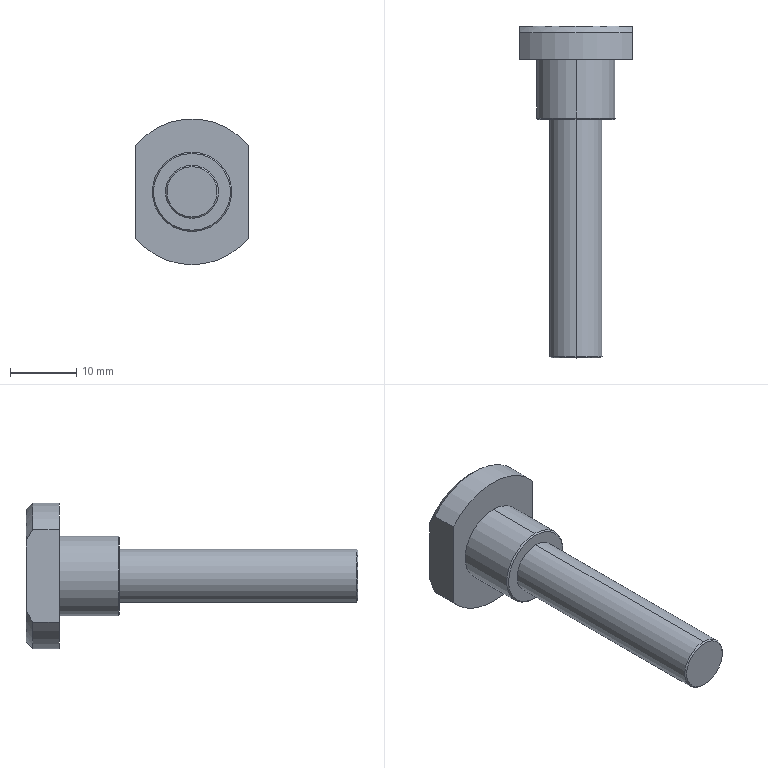Part | STEP file | BPSP-11-20 Cylinder Connection Shoulder Screw_Default | 1 solid | 20 faces | box 17 x 50.1 x 22 mm | volume 4480 mm3 | cone 7 | cylinder 7 | plane 6 | commonest cylinder face diameters 22 x3 8 x2 12 x2
STEP:
#1=CARTESIAN_POINT('',(0.,0.,0.));
#2=DIRECTION('',(0.,0.,1.));
#3=DIRECTION('',(1.,0.,0.));
#4=AXIS2_PLACEMENT_3D('',#1,#2,#3);
#5=CARTESIAN_POINT('',(0.,0.,-3.8));
#6=VERTEX_POINT('',#5);
#7=CARTESIAN_POINT('',(0.,0.,3.8));
#8=VERTEX_POINT('',#7);
#9=CARTESIAN_POINT('',(0.,0.,0.));
#10=DIRECTION('',(0.,-1.,0.));
#11=DIRECTION('',(0.,0.,1.));
#12=AXIS2_PLACEMENT_3D('',#9,#10,#11);
#13=CIRCLE('',#12,3.8);
#14=CARTESIAN_POINT('',(0.,0.2,0.));
#15=DIRECTION('',(0.,1.,0.));
#16=DIRECTION('',(0.,0.,1.));
#17=AXIS2_PLACEMENT_3D('',#14,#15,#16);
#18=CONICAL_SURFACE('',#17,4.,0.7854);
#19=CARTESIAN_POINT('',(6.283,-0.2));
#20=DIRECTION('',(-1.,0.));
#21=VECTOR('',#20,1.);
#22=LINE('',#19,#21);
#23=(GEOMETRIC_REPRESENTATION_CONTEXT(2)PARAMETRIC_REPRESENTATION_CONTEXT()REPRESENTATION_CONTEXT('',''));
#24=DEFINITIONAL_REPRESENTATION('',(#22),#23);
#25=PCURVE('',#18,#24);
#26=CARTESIAN_POINT('',(0.,0.,0.));
#27=DIRECTION('',(0.,1.,0.));
#28=DIRECTION('',(0.,0.,1.));
#29=AXIS2_PLACEMENT_3D('',#26,#27,#28);
#30=PLANE('',#29);
#31=CARTESIAN_POINT('',(3.8,0.));
#32=CARTESIAN_POINT('',(3.8,-6.582));
#33=CARTESIAN_POINT('',(-1.9,-3.291));
#34=CARTESIAN_POINT('',(-7.6,0.));
#35=CARTESIAN_POINT('',(-1.9,3.291));
#36=CARTESIAN_POINT('',(3.8,6.582));
#37=CARTESIAN_POINT('',(3.8,0.));
#38=(BOUNDED_CURVE()B_SPLINE_CURVE(2,(#31,#32,#33,#34,#35,#36,#37),.UNSPECIFIED.,.T.,.F.)B_SPLINE_CURVE_WITH_KNOTS((1,2,2,2,2,1),(-2.094,0.,2.094,4.189,6.283,8.378),.UNSPECIFIED.)CURVE()GEOMETRIC_REPRESENTATION_ITEM()RATIONAL_B_SPLINE_CURVE((1.,0.5,1.,0.5,1.,0.5,1.))REPRESENTATION_ITEM(''));
#39=(GEOMETRIC_REPRESENTATION_CONTEXT(2)PARAMETRIC_REPRESENTATION_CONTEXT()REPRESENTATION_CONTEXT('',''));
#40=DEFINITIONAL_REPRESENTATION('',(#38),#39);
#41=PCURVE('',#30,#40);
#42=SURFACE_CURVE('',#13,(#25,#41),.PCURVE_S1.);
#43=EDGE_CURVE('',#6,#8,#42,.T.);
#44=ORIENTED_EDGE('',*,*,#43,.F.);
#45=CARTESIAN_POINT('',(0.,0.2,-4.));
#46=VERTEX_POINT('',#45);
#47=CARTESIAN_POINT('',(0.,0.2,-4.));
#48=DIRECTION('',(0.,0.7071,-0.7071));
#49=VECTOR('',#48,1.);
#50=LINE('',#47,#49);
#51=CARTESIAN_POINT('',(3.142,0.));
#52=DIRECTION('',(0.,1.));
#53=VECTOR('',#52,1.);
#54=LINE('',#51,#53);
#55=(GEOMETRIC_REPRESENTATION_CONTEXT(2)PARAMETRIC_REPRESENTATION_CONTEXT()REPRESENTATION_CONTEXT('',''));
#56=DEFINITIONAL_REPRESENTATION('',(#54),#55);
#57=PCURVE('',#18,#56);
#58=CARTESIAN_POINT('',(0.,0.2,0.));
#59=DIRECTION('',(0.,1.,0.));
#60=DIRECTION('',(0.,0.,1.));
#61=AXIS2_PLACEMENT_3D('',#58,#59,#60);
#62=CONICAL_SURFACE('',#61,4.,0.7854);
#63=CARTESIAN_POINT('',(3.142,0.));
#64=DIRECTION('',(0.,1.));
#65=VECTOR('',#64,1.);
#66=LINE('',#63,#65);
#67=(GEOMETRIC_REPRESENTATION_CONTEXT(2)PARAMETRIC_REPRESENTATION_CONTEXT()REPRESENTATION_CONTEXT('',''));
#68=DEFINITIONAL_REPRESENTATION('',(#66),#67);
#69=PCURVE('',#62,#68);
#70=SURFACE_CURVE('',#50,(#57,#69),.PCURVE_S1.);
#71=EDGE_CURVE('',#6,#46,#70,.T.);
#72=ORIENTED_EDGE('',*,*,#71,.T.);
#73=CARTESIAN_POINT('',(0.,0.2,4.));
#74=VERTEX_POINT('',#73);
#75=CARTESIAN_POINT('',(0.,0.2,0.));
#76=DIRECTION('',(0.,1.,0.));
#77=DIRECTION('',(0.,0.,1.));
#78=AXIS2_PLACEMENT_3D('',#75,#76,#77);
#79=CIRCLE('',#78,4.);
#80=CARTESIAN_POINT('',(0.,0.));
#81=DIRECTION('',(1.,0.));
#82=VECTOR('',#81,1.);
#83=LINE('',#80,#82);
#84=(GEOMETRIC_REPRESENTATION_CONTEXT(2)PARAMETRIC_REPRESENTATION_CONTEXT()REPRESENTATION_CONTEXT('',''));
#85=DEFINITIONAL_REPRESENTATION('',(#83),#84);
#86=PCURVE('',#18,#85);
#87=CARTESIAN_POINT('',(0.,36.,0.));
#88=DIRECTION('',(0.,-1.,0.));
#89=DIRECTION('',(0.,0.,-1.));
#90=AXIS2_PLACEMENT_3D('',#87,#88,#89);
#91=CYLINDRICAL_SURFACE('',#90,4.);
#92=CARTESIAN_POINT('',(3.142,35.8));
#93=DIRECTION('',(-1.,0.));
#94=VECTOR('',#93,1.);
#95=LINE('',#92,#94);
#96=(GEOMETRIC_REPRESENTATION_CONTEXT(2)PARAMETRIC_REPRESENTATION_CONTEXT()REPRESENTATION_CONTEXT('',''));
#97=DEFINITIONAL_REPRESENTATION('',(#95),#96);
#98=PCURVE('',#91,#97);
#99=SURFACE_CURVE('',#79,(#86,#98),.PCURVE_S1.);
#100=EDGE_CURVE('',#74,#46,#99,.T.);
#101=ORIENTED_EDGE('',*,*,#100,.F.);
#102=CARTESIAN_POINT('',(0.,0.2,4.));
#103=DIRECTION('',(0.,0.7071,0.7071));
#104=VECTOR('',#103,1.);
#105=LINE('',#102,#104);
#106=CARTESIAN_POINT('',(0.,0.));
#107=DIRECTION('',(0.,1.));
#108=VECTOR('',#107,1.);
#109=LINE('',#106,#108);
#110=(GEOMETRIC_REPRESENTATION_CONTEXT(2)PARAMETRIC_REPRESENTATION_CONTEXT()REPRESENTATION_CONTEXT('',''));
#111=DEFINITIONAL_REPRESENTATION('',(#109),#110);
#112=PCURVE('',#18,#111);
#113=CARTESIAN_POINT('',(6.283,0.));
#114=DIRECTION('',(0.,1.));
#115=VECTOR('',#114,1.);
#116=LINE('',#113,#115);
#117=(GEOMETRIC_REPRESENTATION_CONTEXT(2)PARAMETRIC_REPRESENTATION_CONTEXT()REPRESENTATION_CONTEXT('',''));
#118=DEFINITIONAL_REPRESENTATION('',(#116),#117);
#119=PCURVE('',#62,#118);
#120=SURFACE_CURVE('',#105,(#112,#119),.PCURVE_S1.);
#121=EDGE_CURVE('',#8,#74,#120,.T.);
#122=ORIENTED_EDGE('',*,*,#121,.F.);
#123=EDGE_LOOP('',(#44,#72,#101,#122));
#124=FACE_BOUND('',#123,.T.);
#125=ADVANCED_FACE('',(#124),#18,.T.);
#126=CARTESIAN_POINT('',(0.,36.,-5.8));
#127=VERTEX_POINT('',#126);
#128=CARTESIAN_POINT('',(0.,36.,5.8));
#129=VERTEX_POINT('',#128);
#130=CARTESIAN_POINT('',(0.,36.,0.));
#131=DIRECTION('',(0.,-1.,0.));
#132=DIRECTION('',(0.,0.,1.));
#133=AXIS2_PLACEMENT_3D('',#130,#131,#132);
#134=CIRCLE('',#133,5.8);
#135=CARTESIAN_POINT('',(0.,36.2,0.));
#136=DIRECTION('',(0.,1.,0.));
#137=DIRECTION('',(0.,0.,1.));
#138=AXIS2_PLACEMENT_3D('',#135,#136,#137);
#139=CONICAL_SURFACE('',#138,6.,0.7854);
#140=CARTESIAN_POINT('',(6.283,-0.2));
#141=DIRECTION('',(-1.,0.));
#142=VECTOR('',#141,1.);
#143=LINE('',#140,#142);
#144=(GEOMETRIC_REPRESENTATION_CONTEXT(2)PARAMETRIC_REPRESENTATION_CONTEXT()REPRESENTATION_CONTEXT('',''));
#145=DEFINITIONAL_REPRESENTATION('',(#143),#144);
#146=PCURVE('',#139,#145);
#147=CARTESIAN_POINT('',(0.,36.,0.));
#148=DIRECTION('',(0.,1.,0.));
#149=DIRECTION('',(0.,0.,1.));
#150=AXIS2_PLACEMENT_3D('',#147,#148,#149);
#151=PLANE('',#150);
#152=CARTESIAN_POINT('',(5.8,0.));
#153=CARTESIAN_POINT('',(5.8,-10.046));
#154=CARTESIAN_POINT('',(-2.9,-5.023));
#155=CARTESIAN_POINT('',(-11.6,0.));
#156=CARTESIAN_POINT('',(-2.9,5.023));
#157=CARTESIAN_POINT('',(5.8,10.046));
#158=CARTESIAN_POINT('',(5.8,0.));
#159=(BOUNDED_CURVE()B_SPLINE_CURVE(2,(#152,#153,#154,#155,#156,#157,#158),.UNSPECIFIED.,.T.,.F.)B_SPLINE_CURVE_WITH_KNOTS((1,2,2,2,2,1),(-2.094,0.,2.094,4.189,6.283,8.378),.UNSPECIFIED.)CURVE()GEOMETRIC_REPRESENTATION_ITEM()RATIONAL_B_SPLINE_CURVE((1.,0.5,1.,0.5,1.,0.5,1.))REPRESENTATION_ITEM(''));
#160=(GEOMETRIC_REPRESENTATION_CONTEXT(2)PARAMETRIC_REPRESENTATION_CONTEXT()REPRESENTATION_CONTEXT('',''));
#161=DEFINITIONAL_REPRESENTATION('',(#159),#160);
#162=PCURVE('',#151,#161);
#163=SURFACE_CURVE('',#134,(#146,#162),.PCURVE_S1.);
#164=EDGE_CURVE('',#127,#129,#163,.T.);
#165=ORIENTED_EDGE('',*,*,#164,.F.);
#166=CARTESIAN_POINT('',(0.,36.2,-6.));
#167=VERTEX_POINT('',#166);
#168=CARTESIAN_POINT('',(0.,36.2,-6.));
#169=DIRECTION('',(0.,0.7071,-0.7071));
#170=VECTOR('',#169,1.);
#171=LINE('',#168,#170);
#172=CARTESIAN_POINT('',(3.142,0.));
#173=DIRECTION('',(0.,1.));
#174=VECTOR('',#173,1.);
#175=LINE('',#172,#174);
#176=(GEOMETRIC_REPRESENTATION_CONTEXT(2)PARAMETRIC_REPRESENTATION_CONTEXT()REPRESENTATION_CONTEXT('',''));
#177=DEFINITIONAL_REPRESENTATION('',(#175),#176);
#178=PCURVE('',#139,#177);
#179=CARTESIAN_POINT('',(0.,36.2,0.));
#180=DIRECTION('',(0.,1.,0.));
#181=DIRECTION('',(0.,0.,1.));
#182=AXIS2_PLACEMENT_3D('',#179,#180,#181);
#183=CONICAL_SURFACE('',#182,6.,0.7854);
#184=CARTESIAN_POINT('',(3.142,0.));
#185=DIRECTION('',(0.,1.));
#186=VECTOR('',#185,1.);
#187=LINE('',#184,#186);
#188=(GEOMETRIC_REPRESENTATION_CONTEXT(2)PARAMETRIC_REPRESENTATION_CONTEXT()REPRESENTATION_CONTEXT('',''));
#189=DEFINITIONAL_REPRESENTATION('',(#187),#188);
#190=PCURVE('',#183,#189);
#191=SURFACE_CURVE('',#171,(#178,#190),.PCURVE_S1.);
#192=EDGE_CURVE('',#127,#167,#191,.T.);
#193=ORIENTED_EDGE('',*,*,#192,.T.);
#194=CARTESIAN_POINT('',(0.,36.2,6.));
#195=VERTEX_POINT('',#194);
#196=CARTESIAN_POINT('',(0.,36.2,0.));
#197=DIRECTION('',(0.,1.,0.));
#198=DIRECTION('',(0.,0.,1.));
#199=AXIS2_PLACEMENT_3D('',#196,#197,#198);
#200=CIRCLE('',#199,6.);
#201=CARTESIAN_POINT('',(0.,0.));
#202=DIRECTION('',(1.,0.));
#203=VECTOR('',#202,1.);
#204=LINE('',#201,#203);
#205=(GEOMETRIC_REPRESENTATION_CONTEXT(2)PARAMETRIC_REPRESENTATION_CONTEXT()REPRESENTATION_CONTEXT('',''));
#206=DEFINITIONAL_REPRESENTATION('',(#204),#205);
#207=PCURVE('',#139,#206);
#208=CARTESIAN_POINT('',(0.,45.1,0.));
#209=DIRECTION('',(0.,-1.,0.));
#210=DIRECTION('',(0.,0.,-1.));
#211=AXIS2_PLACEMENT_3D('',#208,#209,#210);
#212=CYLINDRICAL_SURFACE('',#211,6.);
#213=CARTESIAN_POINT('',(3.142,8.9));
#214=DIRECTION('',(-1.,0.));
#215=VECTOR('',#214,1.);
#216=LINE('',#213,#215);
#217=(GEOMETRIC_REPRESENTATION_CONTEXT(2)PARAMETRIC_REPRESENTATION_CONTEXT()REPRESENTATION_CONTEXT('',''));
#218=DEFINITIONAL_REPRESENTATION('',(#216),#217);
#219=PCURVE('',#212,#218);
#220=SURFACE_CURVE('',#200,(#207,#219),.PCURVE_S1.);
#221=EDGE_CURVE('',#195,#167,#220,.T.);
#222=ORIENTED_EDGE('',*,*,#221,.F.);
#223=CARTESIAN_POINT('',(0.,36.2,6.));
#224=DIRECTION('',(0.,0.7071,0.7071));
#225=VECTOR('',#224,1.);
#226=LINE('',#223,#225);
#227=CARTESIAN_POINT('',(0.,0.));
#228=DIRECTION('',(0.,1.));
#229=VECTOR('',#228,1.);
#230=LINE('',#227,#229);
#231=(GEOMETRIC_REPRESENTATION_CONTEXT(2)PARAMETRIC_REPRESENTATION_CONTEXT()REPRESENTATION_CONTEXT('',''));
#232=DEFINITIONAL_REPRESENTATION('',(#230),#231);
#233=PCURVE('',#139,#232);
#234=CARTESIAN_POINT('',(6.283,0.));
#235=DIRECTION('',(0.,1.));
#236=VECTOR('',#235,1.);
#237=LINE('',#234,#236);
#238=(GEOMETRIC_REPRESENTATION_CONTEXT(2)PARAMETRIC_REPRESENTATION_CONTEXT()REPRESENTATION_CONTEXT('',''));
#239=DEFINITIONAL_REPRESENTATION('',(#237),#238);
#240=PCURVE('',#183,#239);
#241=SURFACE_CURVE('',#226,(#233,#240),.PCURVE_S1.);
#242=EDGE_CURVE('',#129,#195,#241,.T.);
#243=ORIENTED_EDGE('',*,*,#242,.F.);
#244=EDGE_LOOP('',(#165,#193,#222,#243));
#245=FACE_BOUND('',#244,.T.);
#246=ADVANCED_FACE('',(#245),#139,.T.);
#247=CARTESIAN_POINT('',(0.,50.1,-10.));
#248=VERTEX_POINT('',#247);
#249=CARTESIAN_POINT('',(-8.5,50.1,-5.268));
#250=VERTEX_POINT('',#249);
#251=CARTESIAN_POINT('',(0.,50.1,0.));
#252=DIRECTION('',(0.,1.,0.));
#253=DIRECTION('',(0.,0.,1.));
#254=AXIS2_PLACEMENT_3D('',#251,#252,#253);
#255=CIRCLE('',#254,10.);
#256=CARTESIAN_POINT('',(0.,50.1,0.));
#257=DIRECTION('',(0.,-1.,0.));
#258=DIRECTION('',(0.,0.,-1.));
#259=AXIS2_PLACEMENT_3D('',#256,#257,#258);
#260=CONICAL_SURFACE('',#259,10.,0.7854);
#261=CARTESIAN_POINT('',(9.425,0.));
#262=DIRECTION('',(-1.,0.));
#263=VECTOR('',#262,1.);
#264=LINE('',#261,#263);
#265=(GEOMETRIC_REPRESENTATION_CONTEXT(2)PARAMETRIC_REPRESENTATION_CONTEXT()REPRESENTATION_CONTEXT('',''));
#266=DEFINITIONAL_REPRESENTATION('',(#264),#265);
#267=PCURVE('',#260,#266);
#268=CARTESIAN_POINT('',(0.,50.1,0.));
#269=DIRECTION('',(0.,1.,0.));
#270=DIRECTION('',(0.,0.,1.));
#271=AXIS2_PLACEMENT_3D('',#268,#269,#270);
#272=PLANE('',#271);
#273=CARTESIAN_POINT('',(0.,0.));
#274=DIRECTION('',(1.,0.));
#275=AXIS2_PLACEMENT_2D('',#273,#274);
#276=CIRCLE('',#275,10.);
#277=(GEOMETRIC_REPRESENTATION_CONTEXT(2)PARAMETRIC_REPRESENTATION_CONTEXT()REPRESENTATION_CONTEXT('',''));
#278=DEFINITIONAL_REPRESENTATION('',(#276),#277);
#279=PCURVE('',#272,#278);
#280=SURFACE_CURVE('',#255,(#267,#279),.PCURVE_S1.);
#281=EDGE_CURVE('',#248,#250,#280,.T.);
#282=ORIENTED_EDGE('',*,*,#281,.F.);
#283=CARTESIAN_POINT('',(0.,49.1,-11.));
#284=VERTEX_POINT('',#283);
#285=CARTESIAN_POINT('',(0.,50.1,-10.));
#286=DIRECTION('',(0.,-0.7071,-0.7071));
#287=VECTOR('',#286,1.);
#288=LINE('',#285,#287);
#289=CARTESIAN_POINT('',(6.283,0.));
#290=DIRECTION('',(0.,1.));
#291=VECTOR('',#290,1.);
#292=LINE('',#289,#291);
#293=(GEOMETRIC_REPRESENTATION_CONTEXT(2)PARAMETRIC_REPRESENTATION_CONTEXT()REPRESENTATION_CONTEXT('',''));
#294=DEFINITIONAL_REPRESENTATION('',(#292),#293);
#295=PCURVE('',#260,#294);
#296=CARTESIAN_POINT('',(0.,50.1,0.));
#297=DIRECTION('',(0.,-1.,0.));
#298=DIRECTION('',(0.,0.,-1.));
#299=AXIS2_PLACEMENT_3D('',#296,#297,#298);
#300=CONICAL_SURFACE('',#299,10.,0.7854);
#301=CARTESIAN_POINT('',(0.,0.));
#302=DIRECTION('',(0.,1.));
#303=VECTOR('',#302,1.);
#304=LINE('',#301,#303);
#305=(GEOMETRIC_REPRESENTATION_CONTEXT(2)PARAMETRIC_REPRESENTATION_CONTEXT()REPRESENTATION_CONTEXT('',''));
#306=DEFINITIONAL_REPRESENTATION('',(#304),#305);
#307=PCURVE('',#300,#306);
#308=SURFACE_CURVE('',#288,(#295,#307),.PCURVE_S1.);
#309=EDGE_CURVE('',#248,#284,#308,.T.);
#310=ORIENTED_EDGE('',*,*,#309,.T.);
#311=CARTESIAN_POINT('',(-8.5,49.1,-6.982));
#312=VERTEX_POINT('',#311);
#313=CARTESIAN_POINT('',(0.,49.1,0.));
#314=DIRECTION('',(0.,-1.,0.));
#315=DIRECTION('',(0.,0.,1.));
#316=AXIS2_PLACEMENT_3D('',#313,#314,#315);
#317=CIRCLE('',#316,11.);
#318=CARTESIAN_POINT('',(3.142,1.));
#319=DIRECTION('',(1.,0.));
#320=VECTOR('',#319,1.);
#321=LINE('',#318,#320);
#322=(GEOMETRIC_REPRESENTATION_CONTEXT(2)PARAMETRIC_REPRESENTATION_CONTEXT()REPRESENTATION_CONTEXT('',''));
#323=DEFINITIONAL_REPRESENTATION('',(#321),#322);
#324=PCURVE('',#260,#323);
#325=CARTESIAN_POINT('',(0.,50.1,0.));
#326=DIRECTION('',(0.,-1.,0.));
#327=DIRECTION('',(0.,0.,-1.));
#328=AXIS2_PLACEMENT_3D('',#325,#326,#327);
#329=CYLINDRICAL_SURFACE('',#328,11.);
#330=CARTESIAN_POINT('',(3.142,1.));
#331=DIRECTION('',(1.,0.));
#332=VECTOR('',#331,1.);
#333=LINE('',#330,#332);
#334=(GEOMETRIC_REPRESENTATION_CONTEXT(2)PARAMETRIC_REPRESENTATION_CONTEXT()REPRESENTATION_CONTEXT('',''));
#335=DEFINITIONAL_REPRESENTATION('',(#333),#334);
#336=PCURVE('',#329,#335);
#337=SURFACE_CURVE('',#317,(#324,#336),.PCURVE_S1.);
#338=EDGE_CURVE('',#312,#284,#337,.T.);
#339=ORIENTED_EDGE('',*,*,#338,.F.);
#340=CARTESIAN_POINT('',(-8.5,50.1,-5.268));
#341=CARTESIAN_POINT('',(-8.5,49.791,-5.854));
#342=CARTESIAN_POINT('',(-8.5,49.455,-6.423));
#343=CARTESIAN_POINT('',(-8.5,49.1,-6.982));
#344=B_SPLINE_CURVE_WITH_KNOTS('',3,(#340,#341,#342,#343),.UNSPECIFIED.,.F.,.F.,(4,4),(0.,0.001985),.PIECEWISE_BEZIER_KNOTS.);
#345=CARTESIAN_POINT('',(5.267,0.));
#346=CARTESIAN_POINT('',(5.269,0.01403));
#347=CARTESIAN_POINT('',(5.274,0.0422));
#348=CARTESIAN_POINT('',(5.281,0.0848));
#349=CARTESIAN_POINT('',(5.287,0.1277));
#350=CARTESIAN_POINT('',(5.294,0.171));
#351=CARTESIAN_POINT('',(5.3,0.2146));
#352=CARTESIAN_POINT('',(5.307,0.2585));
#353=CARTESIAN_POINT('',(5.313,0.3028));
#354=CARTESIAN_POINT('',(5.319,0.3473));
#355=CARTESIAN_POINT('',(5.325,0.3921));
#356=CARTESIAN_POINT('',(5.332,0.4373));
#357=CARTESIAN_POINT('',(5.338,0.4827));
#358=CARTESIAN_POINT('',(5.344,0.5284));
#359=CARTESIAN_POINT('',(5.35,0.5744));
#360=CARTESIAN_POINT('',(5.355,0.6207));
#361=CARTESIAN_POINT('',(5.361,0.6672));
#362=CARTESIAN_POINT('',(5.367,0.714));
#363=CARTESIAN_POINT('',(5.373,0.761));
#364=CARTESIAN_POINT('',(5.378,0.8083));
#365=CARTESIAN_POINT('',(5.384,0.8559));
#366=CARTESIAN_POINT('',(5.389,0.9037));
#367=CARTESIAN_POINT('',(5.395,0.9517));
#368=CARTESIAN_POINT('',(5.398,0.9839));
#369=CARTESIAN_POINT('',(5.4,1.));
#370=B_SPLINE_CURVE_WITH_KNOTS('',3,(#345,#346,#347,#348,#349,#350,#351,#352,#353,#354,#355,#356,#357,#358,#359,#360,#361,#362,#363,#364,#365,#366,#367,#368,#369),.UNSPECIFIED.,.F.,.F.,(4,1,1,1,1,1,1,1,1,1,1,1,1,1,1,1,1,1,1,1,1,1,4),(0.,0.00009021,0.0001804,0.0002706,0.0003608,0.0004511,0.0005413,0.0006315,0.0007217,0.0008119,0.0009021,0.0009923,0.001083,0.001173,0.001263,0.001353,0.001443,0.001534,0.001624,0.001714,0.001804,0.001894,0.001985),.QUASI_UNIFORM_KNOTS.);
#371=(GEOMETRIC_REPRESENTATION_CONTEXT(2)PARAMETRIC_REPRESENTATION_CONTEXT()REPRESENTATION_CONTEXT('',''));
#372=DEFINITIONAL_REPRESENTATION('',(#370),#371);
#373=PCURVE('',#260,#372);
#374=CARTESIAN_POINT('',(-8.5,0.,-13.972));
#375=DIRECTION('',(-1.,0.,0.));
#376=DIRECTION('',(0.,0.,1.));
#377=AXIS2_PLACEMENT_3D('',#374,#375,#376);
#378=PLANE('',#377);
#379=CARTESIAN_POINT('',(8.705,50.1));
#380=CARTESIAN_POINT('',(8.119,49.791));
#381=CARTESIAN_POINT('',(7.549,49.455));
#382=CARTESIAN_POINT('',(6.99,49.1));
#383=B_SPLINE_CURVE_WITH_KNOTS('',3,(#379,#380,#381,#382),.UNSPECIFIED.,.F.,.F.,(4,4),(0.,0.001985),.PIECEWISE_BEZIER_KNOTS.);
#384=(GEOMETRIC_REPRESENTATION_CONTEXT(2)PARAMETRIC_REPRESENTATION_CONTEXT()REPRESENTATION_CONTEXT('',''));
#385=DEFINITIONAL_REPRESENTATION('',(#383),#384);
#386=PCURVE('',#378,#385);
#387=SURFACE_CURVE('',#344,(#373,#386),.PCURVE_S1.);
#388=EDGE_CURVE('',#250,#312,#387,.T.);
#389=ORIENTED_EDGE('',*,*,#388,.F.);
#390=EDGE_LOOP('',(#282,#310,#339,#389));
#391=FACE_BOUND('',#390,.T.);
#392=ADVANCED_FACE('',(#391),#260,.T.);
#393=CARTESIAN_POINT('',(0.,45.1,6.));
#394=VERTEX_POINT('',#393);
#395=CARTESIAN_POINT('',(0.,45.1,-6.));
#396=VERTEX_POINT('',#395);
#397=CARTESIAN_POINT('',(0.,45.1,0.));
#398=DIRECTION('',(0.,1.,0.));
#399=DIRECTION('',(0.,0.,1.));
#400=AXIS2_PLACEMENT_3D('',#397,#398,#399);
#401=CIRCLE('',#400,6.);
#402=CARTESIAN_POINT('',(3.142,0.));
#403=DIRECTION('',(-1.,0.));
#404=VECTOR('',#403,1.);
#405=LINE('',#402,#404);
#406=(GEOMETRIC_REPRESENTATION_CONTEXT(2)PARAMETRIC_REPRESENTATION_CONTEXT()REPRESENTATION_CONTEXT('',''));
#407=DEFINITIONAL_REPRESENTATION('',(#405),#406);
#408=PCURVE('',#212,#407);
#409=CARTESIAN_POINT('',(0.,45.1,0.));
#410=DIRECTION('',(0.,1.,0.));
#411=DIRECTION('',(0.,0.,1.));
#412=AXIS2_PLACEMENT_3D('',#409,#410,#411);
#413=PLANE('',#412);
#414=CARTESIAN_POINT('',(0.,0.));
#415=DIRECTION('',(1.,0.));
#416=AXIS2_PLACEMENT_2D('',#414,#415);
#417=CIRCLE('',#416,6.);
#418=(GEOMETRIC_REPRESENTATION_CONTEXT(2)PARAMETRIC_REPRESENTATION_CONTEXT()REPRESENTATION_CONTEXT('',''));
#419=DEFINITIONAL_REPRESENTATION('',(#417),#418);
#420=PCURVE('',#413,#419);
#421=SURFACE_CURVE('',#401,(#408,#420),.PCURVE_S1.);
#422=EDGE_CURVE('',#394,#396,#421,.T.);
#423=ORIENTED_EDGE('',*,*,#422,.F.);
#424=CARTESIAN_POINT('',(0.,45.1,6.));
#425=DIRECTION('',(0.,-1.,0.));
#426=VECTOR('',#425,1.);
#427=LINE('',#424,#426);
#428=CARTESIAN_POINT('',(3.142,0.));
#429=DIRECTION('',(0.,1.));
#430=VECTOR('',#429,1.);
#431=LINE('',#428,#430);
#432=(GEOMETRIC_REPRESENTATION_CONTEXT(2)PARAMETRIC_REPRESENTATION_CONTEXT()REPRESENTATION_CONTEXT('',''));
#433=DEFINITIONAL_REPRESENTATION('',(#431),#432);
#434=PCURVE('',#212,#433);
#435=CARTESIAN_POINT('',(0.,45.1,0.));
#436=DIRECTION('',(0.,-1.,0.));
#437=DIRECTION('',(0.,0.,-1.));
#438=AXIS2_PLACEMENT_3D('',#435,#436,#437);
#439=CYLINDRICAL_SURFACE('',#438,6.);
#440=CARTESIAN_POINT('',(3.142,0.));
#441=DIRECTION('',(0.,1.));
#442=VECTOR('',#441,1.);
#443=LINE('',#440,#442);
#444=(GEOMETRIC_REPRESENTATION_CONTEXT(2)PARAMETRIC_REPRESENTATION_CONTEXT()REPRESENTATION_CONTEXT('',''));
#445=DEFINITIONAL_REPRESENTATION('',(#443),#444);
#446=PCURVE('',#439,#445);
#447=SURFACE_CURVE('',#427,(#434,#446),.PCURVE_S1.);
#448=EDGE_CURVE('',#394,#195,#447,.T.);
#449=ORIENTED_EDGE('',*,*,#448,.T.);
#450=ORIENTED_EDGE('',*,*,#221,.T.);
#451=CARTESIAN_POINT('',(0.,45.1,-6.));
#452=DIRECTION('',(0.,-1.,0.));
#453=VECTOR('',#452,1.);
#454=LINE('',#451,#453);
#455=CARTESIAN_POINT('',(0.,0.));
#456=DIRECTION('',(0.,1.));
#457=VECTOR('',#456,1.);
#458=LINE('',#455,#457);
#459=(GEOMETRIC_REPRESENTATION_CONTEXT(2)PARAMETRIC_REPRESENTATION_CONTEXT()REPRESENTATION_CONTEXT('',''));
#460=DEFINITIONAL_REPRESENTATION('',(#458),#459);
#461=PCURVE('',#212,#460);
#462=CARTESIAN_POINT('',(6.283,0.));
#463=DIRECTION('',(0.,1.));
#464=VECTOR('',#463,1.);
#465=LINE('',#462,#464);
#466=(GEOMETRIC_REPRESENTATION_CONTEXT(2)PARAMETRIC_REPRESENTATION_CONTEXT()REPRESENTATION_CONTEXT('',''));
#467=DEFINITIONAL_REPRESENTATION('',(#465),#466);
#468=PCURVE('',#439,#467);
#469=SURFACE_CURVE('',#454,(#461,#468),.PCURVE_S1.);
#470=EDGE_CURVE('',#396,#167,#469,.T.);
#471=ORIENTED_EDGE('',*,*,#470,.F.);
#472=EDGE_LOOP('',(#423,#449,#450,#471));
#473=FACE_BOUND('',#472,.T.);
#474=ADVANCED_FACE('',(#473),#212,.T.);
#475=CARTESIAN_POINT('',(0.,36.,4.));
#476=VERTEX_POINT('',#475);
#477=CARTESIAN_POINT('',(0.,36.,-4.));
#478=VERTEX_POINT('',#477);
#479=CARTESIAN_POINT('',(0.,36.,0.));
#480=DIRECTION('',(0.,1.,0.));
#481=DIRECTION('',(0.,0.,1.));
#482=AXIS2_PLACEMENT_3D('',#479,#480,#481);
#483=CIRCLE('',#482,4.);
#484=CARTESIAN_POINT('',(3.142,0.));
#485=DIRECTION('',(-1.,0.));
#486=VECTOR('',#485,1.);
#487=LINE('',#484,#486);
#488=(GEOMETRIC_REPRESENTATION_CONTEXT(2)PARAMETRIC_REPRESENTATION_CONTEXT()REPRESENTATION_CONTEXT('',''));
#489=DEFINITIONAL_REPRESENTATION('',(#487),#488);
#490=PCURVE('',#91,#489);
#491=CARTESIAN_POINT('',(0.,0.));
#492=DIRECTION('',(1.,0.));
#493=AXIS2_PLACEMENT_2D('',#491,#492);
#494=CIRCLE('',#493,4.);
#495=(GEOMETRIC_REPRESENTATION_CONTEXT(2)PARAMETRIC_REPRESENTATION_CONTEXT()REPRESENTATION_CONTEXT('',''));
#496=DEFINITIONAL_REPRESENTATION('',(#494),#495);
#497=PCURVE('',#151,#496);
#498=SURFACE_CURVE('',#483,(#490,#497),.PCURVE_S1.);
#499=EDGE_CURVE('',#476,#478,#498,.T.);
#500=ORIENTED_EDGE('',*,*,#499,.F.);
#501=CARTESIAN_POINT('',(0.,36.,4.));
#502=DIRECTION('',(0.,-1.,0.));
#503=VECTOR('',#502,1.);
#504=LINE('',#501,#503);
#505=CARTESIAN_POINT('',(3.142,0.));
#506=DIRECTION('',(0.,1.));
#507=VECTOR('',#506,1.);
#508=LINE('',#505,#507);
#509=(GEOMETRIC_REPRESENTATION_CONTEXT(2)PARAMETRIC_REPRESENTATION_CONTEXT()REPRESENTATION_CONTEXT('',''));
#510=DEFINITIONAL_REPRESENTATION('',(#508),#509);
#511=PCURVE('',#91,#510);
#512=CARTESIAN_POINT('',(0.,36.,0.));
#513=DIRECTION('',(0.,-1.,0.));
#514=DIRECTION('',(0.,0.,-1.));
#515=AXIS2_PLACEMENT_3D('',#512,#513,#514);
#516=CYLINDRICAL_SURFACE('',#515,4.);
#517=CARTESIAN_POINT('',(3.142,0.));
#518=DIRECTION('',(0.,1.));
#519=VECTOR('',#518,1.);
#520=LINE('',#517,#519);
#521=(GEOMETRIC_REPRESENTATION_CONTEXT(2)PARAMETRIC_REPRESENTATION_CONTEXT()REPRESENTATION_CONTEXT('',''));
#522=DEFINITIONAL_REPRESENTATION('',(#520),#521);
#523=PCURVE('',#516,#522);
#524=SURFACE_CURVE('',#504,(#511,#523),.PCURVE_S1.);
#525=EDGE_CURVE('',#476,#74,#524,.T.);
#526=ORIENTED_EDGE('',*,*,#525,.T.);
#527=ORIENTED_EDGE('',*,*,#100,.T.);
#528=CARTESIAN_POINT('',(0.,36.,-4.));
#529=DIRECTION('',(0.,-1.,0.));
#530=VECTOR('',#529,1.);
#531=LINE('',#528,#530);
#532=CARTESIAN_POINT('',(0.,0.));
#533=DIRECTION('',(0.,1.));
#534=VECTOR('',#533,1.);
#535=LINE('',#532,#534);
#536=(GEOMETRIC_REPRESENTATION_CONTEXT(2)PARAMETRIC_REPRESENTATION_CONTEXT()REPRESENTATION_CONTEXT('',''));
#537=DEFINITIONAL_REPRESENTATION('',(#535),#536);
#538=PCURVE('',#91,#537);
#539=CARTESIAN_POINT('',(6.283,0.));
#540=DIRECTION('',(0.,1.));
#541=VECTOR('',#540,1.);
#542=LINE('',#539,#541);
#543=(GEOMETRIC_REPRESENTATION_CONTEXT(2)PARAMETRIC_REPRESENTATION_CONTEXT()REPRESENTATION_CONTEXT('',''));
#544=DEFINITIONAL_REPRESENTATION('',(#542),#543);
#545=PCURVE('',#516,#544);
#546=SURFACE_CURVE('',#531,(#538,#545),.PCURVE_S1.);
#547=EDGE_CURVE('',#478,#46,#546,.T.);
#548=ORIENTED_EDGE('',*,*,#547,.F.);
#549=EDGE_LOOP('',(#500,#526,#527,#548));
#550=FACE_BOUND('',#549,.T.);
#551=ADVANCED_FACE('',(#550),#91,.T.);
#552=ORIENTED_EDGE('',*,*,#338,.T.);
#553=CARTESIAN_POINT('',(0.,45.1,-11.));
#554=VERTEX_POINT('',#553);
#555=CARTESIAN_POINT('',(0.,50.1,-11.));
#556=DIRECTION('',(0.,-1.,0.));
#557=VECTOR('',#556,1.);
#558=LINE('',#555,#557);
#559=CARTESIAN_POINT('',(6.283,0.));
#560=DIRECTION('',(0.,1.));
#561=VECTOR('',#560,1.);
#562=LINE('',#559,#561);
#563=(GEOMETRIC_REPRESENTATION_CONTEXT(2)PARAMETRIC_REPRESENTATION_CONTEXT()REPRESENTATION_CONTEXT('',''));
#564=DEFINITIONAL_REPRESENTATION('',(#562),#563);
#565=PCURVE('',#329,#564);
#566=CARTESIAN_POINT('',(0.,50.1,0.));
#567=DIRECTION('',(0.,-1.,0.));
#568=DIRECTION('',(0.,0.,-1.));
#569=AXIS2_PLACEMENT_3D('',#566,#567,#568);
#570=CYLINDRICAL_SURFACE('',#569,11.);
#571=CARTESIAN_POINT('',(0.,0.));
#572=DIRECTION('',(0.,1.));
#573=VECTOR('',#572,1.);
#574=LINE('',#571,#573);
#575=(GEOMETRIC_REPRESENTATION_CONTEXT(2)PARAMETRIC_REPRESENTATION_CONTEXT()REPRESENTATION_CONTEXT('',''));
#576=DEFINITIONAL_REPRESENTATION('',(#574),#575);
#577=PCURVE('',#570,#576);
#578=SURFACE_CURVE('',#558,(#565,#577),.PCURVE_S1.);
#579=EDGE_CURVE('',#284,#554,#578,.T.);
#580=ORIENTED_EDGE('',*,*,#579,.T.);
#581=CARTESIAN_POINT('',(-8.5,45.1,-6.982));
#582=VERTEX_POINT('',#581);
#583=CARTESIAN_POINT('',(0.,45.1,0.));
#584=DIRECTION('',(0.,1.,0.));
#585=DIRECTION('',(0.,0.,1.));
#586=AXIS2_PLACEMENT_3D('',#583,#584,#585);
#587=CIRCLE('',#586,11.);
#588=CARTESIAN_POINT('',(9.425,5.));
#589=DIRECTION('',(-1.,0.));
#590=VECTOR('',#589,1.);
#591=LINE('',#588,#590);
#592=(GEOMETRIC_REPRESENTATION_CONTEXT(2)PARAMETRIC_REPRESENTATION_CONTEXT()REPRESENTATION_CONTEXT('',''));
#593=DEFINITIONAL_REPRESENTATION('',(#591),#592);
#594=PCURVE('',#329,#593);
#595=CARTESIAN_POINT('',(0.,0.));
#596=DIRECTION('',(1.,0.));
#597=AXIS2_PLACEMENT_2D('',#595,#596);
#598=CIRCLE('',#597,11.);
#599=(GEOMETRIC_REPRESENTATION_CONTEXT(2)PARAMETRIC_REPRESENTATION_CONTEXT()REPRESENTATION_CONTEXT('',''));
#600=DEFINITIONAL_REPRESENTATION('',(#598),#599);
#601=PCURVE('',#413,#600);
#602=SURFACE_CURVE('',#587,(#594,#601),.PCURVE_S1.);
#603=EDGE_CURVE('',#554,#582,#602,.T.);
#604=ORIENTED_EDGE('',*,*,#603,.T.);
#605=CARTESIAN_POINT('',(-8.5,50.1,-6.982));
#606=DIRECTION('',(0.,-1.,0.));
#607=VECTOR('',#606,1.);
#608=LINE('',#605,#607);
#609=CARTESIAN_POINT('',(5.4,0.));
#610=DIRECTION('',(0.,1.));
#611=VECTOR('',#610,1.);
#612=LINE('',#609,#611);
#613=(GEOMETRIC_REPRESENTATION_CONTEXT(2)PARAMETRIC_REPRESENTATION_CONTEXT()REPRESENTATION_CONTEXT('',''));
#614=DEFINITIONAL_REPRESENTATION('',(#612),#613);
#615=PCURVE('',#329,#614);
#616=CARTESIAN_POINT('',(6.99,50.1));
#617=DIRECTION('',(0.,-1.));
#618=VECTOR('',#617,1.);
#619=LINE('',#616,#618);
#620=(GEOMETRIC_REPRESENTATION_CONTEXT(2)PARAMETRIC_REPRESENTATION_CONTEXT()REPRESENTATION_CONTEXT('',''));
#621=DEFINITIONAL_REPRESENTATION('',(#619),#620);
#622=PCURVE('',#378,#621);
#623=SURFACE_CURVE('',#608,(#615,#622),.PCURVE_S1.);
#624=EDGE_CURVE('',#312,#582,#623,.T.);
#625=ORIENTED_EDGE('',*,*,#624,.F.);
#626=EDGE_LOOP('',(#552,#580,#604,#625));
#627=FACE_BOUND('',#626,.T.);
#628=ADVANCED_FACE('',(#627),#329,.T.);
#629=CARTESIAN_POINT('',(0.,45.1,0.));
#630=DIRECTION('',(0.,1.,0.));
#631=DIRECTION('',(0.,0.,1.));
#632=AXIS2_PLACEMENT_3D('',#629,#630,#631);
#633=CIRCLE('',#632,6.);
#634=CARTESIAN_POINT('',(0.,0.));
#635=DIRECTION('',(1.,0.));
#636=AXIS2_PLACEMENT_2D('',#634,#635);
#637=CIRCLE('',#636,6.);
#638=(GEOMETRIC_REPRESENTATION_CONTEXT(2)PARAMETRIC_REPRESENTATION_CONTEXT()REPRESENTATION_CONTEXT('',''));
#639=DEFINITIONAL_REPRESENTATION('',(#637),#638);
#640=PCURVE('',#413,#639);
#641=CARTESIAN_POINT('',(9.425,0.));
#642=DIRECTION('',(-1.,0.));
#643=VECTOR('',#642,1.);
#644=LINE('',#641,#643);
#645=(GEOMETRIC_REPRESENTATION_CONTEXT(2)PARAMETRIC_REPRESENTATION_CONTEXT()REPRESENTATION_CONTEXT('',''));
#646=DEFINITIONAL_REPRESENTATION('',(#644),#645);
#647=PCURVE('',#439,#646);
#648=SURFACE_CURVE('',#633,(#640,#647),.PCURVE_S1.);
#649=EDGE_CURVE('',#396,#394,#648,.T.);
#650=ORIENTED_EDGE('',*,*,#649,.T.);
#651=ORIENTED_EDGE('',*,*,#422,.T.);
#652=EDGE_LOOP('',(#650,#651));
#653=FACE_BOUND('',#652,.T.);
#654=CARTESIAN_POINT('',(8.5,45.1,6.982));
#655=VERTEX_POINT('',#654);
#656=CARTESIAN_POINT('',(8.5,45.1,-6.982));
#657=VERTEX_POINT('',#656);
#658=CARTESIAN_POINT('',(8.5,45.1,0.));
#659=DIRECTION('',(0.,0.,-1.));
#660=VECTOR('',#659,1.);
#661=LINE('',#658,#660);
#662=CARTESIAN_POINT('',(0.,8.5));
#663=DIRECTION('',(-1.,0.));
#664=VECTOR('',#663,1.);
#665=LINE('',#662,#664);
#666=(GEOMETRIC_REPRESENTATION_CONTEXT(2)PARAMETRIC_REPRESENTATION_CONTEXT()REPRESENTATION_CONTEXT('',''));
#667=DEFINITIONAL_REPRESENTATION('',(#665),#666);
#668=PCURVE('',#413,#667);
#669=CARTESIAN_POINT('',(8.5,0.,-13.972));
#670=DIRECTION('',(1.,0.,0.));
#671=DIRECTION('',(0.,0.,-1.));
#672=AXIS2_PLACEMENT_3D('',#669,#670,#671);
#673=PLANE('',#672);
#674=CARTESIAN_POINT('',(-13.972,45.1));
#675=DIRECTION('',(1.,0.));
#676=VECTOR('',#675,1.);
#677=LINE('',#674,#676);
#678=(GEOMETRIC_REPRESENTATION_CONTEXT(2)PARAMETRIC_REPRESENTATION_CONTEXT()REPRESENTATION_CONTEXT('',''));
#679=DEFINITIONAL_REPRESENTATION('',(#677),#678);
#680=PCURVE('',#673,#679);
#681=SURFACE_CURVE('',#661,(#668,#680),.PCURVE_S1.);
#682=EDGE_CURVE('',#655,#657,#681,.T.);
#683=ORIENTED_EDGE('',*,*,#682,.F.);
#684=CARTESIAN_POINT('',(-8.5,45.1,6.982));
#685=VERTEX_POINT('',#684);
#686=CARTESIAN_POINT('',(0.,45.1,0.));
#687=DIRECTION('',(0.,1.,0.));
#688=DIRECTION('',(0.,0.,1.));
#689=AXIS2_PLACEMENT_3D('',#686,#687,#688);
#690=CIRCLE('',#689,11.);
#691=CARTESIAN_POINT('',(0.,0.));
#692=DIRECTION('',(1.,0.));
#693=AXIS2_PLACEMENT_2D('',#691,#692);
#694=CIRCLE('',#693,11.);
#695=(GEOMETRIC_REPRESENTATION_CONTEXT(2)PARAMETRIC_REPRESENTATION_CONTEXT()REPRESENTATION_CONTEXT('',''));
#696=DEFINITIONAL_REPRESENTATION('',(#694),#695);
#697=PCURVE('',#413,#696);
#698=CARTESIAN_POINT('',(0.,50.1,0.));
#699=DIRECTION('',(0.,-1.,0.));
#700=DIRECTION('',(0.,0.,-1.));
#701=AXIS2_PLACEMENT_3D('',#698,#699,#700);
#702=CYLINDRICAL_SURFACE('',#701,11.);
#703=CARTESIAN_POINT('',(9.425,5.));
#704=DIRECTION('',(-1.,0.));
#705=VECTOR('',#704,1.);
#706=LINE('',#703,#705);
#707=(GEOMETRIC_REPRESENTATION_CONTEXT(2)PARAMETRIC_REPRESENTATION_CONTEXT()REPRESENTATION_CONTEXT('',''));
#708=DEFINITIONAL_REPRESENTATION('',(#706),#707);
#709=PCURVE('',#702,#708);
#710=SURFACE_CURVE('',#690,(#697,#709),.PCURVE_S1.);
#711=EDGE_CURVE('',#685,#655,#710,.T.);
#712=ORIENTED_EDGE('',*,*,#711,.F.);
#713=CARTESIAN_POINT('',(-8.5,45.1,0.));
#714=DIRECTION('',(0.,0.,1.));
#715=VECTOR('',#714,1.);
#716=LINE('',#713,#715);
#717=CARTESIAN_POINT('',(0.,-8.5));
#718=DIRECTION('',(1.,0.));
#719=VECTOR('',#718,1.);
#720=LINE('',#717,#719);
#721=(GEOMETRIC_REPRESENTATION_CONTEXT(2)PARAMETRIC_REPRESENTATION_CONTEXT()REPRESENTATION_CONTEXT('',''));
#722=DEFINITIONAL_REPRESENTATION('',(#720),#721);
#723=PCURVE('',#413,#722);
#724=CARTESIAN_POINT('',(13.972,45.1));
#725=DIRECTION('',(1.,0.));
#726=VECTOR('',#725,1.);
#727=LINE('',#724,#726);
#728=(GEOMETRIC_REPRESENTATION_CONTEXT(2)PARAMETRIC_REPRESENTATION_CONTEXT()REPRESENTATION_CONTEXT('',''));
#729=DEFINITIONAL_REPRESENTATION('',(#727),#728);
#730=PCURVE('',#378,#729);
#731=SURFACE_CURVE('',#716,(#723,#730),.PCURVE_S1.);
#732=EDGE_CURVE('',#582,#685,#731,.T.);
#733=ORIENTED_EDGE('',*,*,#732,.F.);
#734=ORIENTED_EDGE('',*,*,#603,.F.);
#735=CARTESIAN_POINT('',(0.,45.1,0.));
#736=DIRECTION('',(0.,1.,0.));
#737=DIRECTION('',(0.,0.,1.));
#738=AXIS2_PLACEMENT_3D('',#735,#736,#737);
#739=CIRCLE('',#738,11.);
#740=CARTESIAN_POINT('',(0.,0.));
#741=DIRECTION('',(1.,0.));
#742=AXIS2_PLACEMENT_2D('',#740,#741);
#743=CIRCLE('',#742,11.);
#744=(GEOMETRIC_REPRESENTATION_CONTEXT(2)PARAMETRIC_REPRESENTATION_CONTEXT()REPRESENTATION_CONTEXT('',''));
#745=DEFINITIONAL_REPRESENTATION('',(#743),#744);
#746=PCURVE('',#413,#745);
#747=CARTESIAN_POINT('',(3.142,5.));
#748=DIRECTION('',(-1.,0.));
#749=VECTOR('',#748,1.);
#750=LINE('',#747,#749);
#751=(GEOMETRIC_REPRESENTATION_CONTEXT(2)PARAMETRIC_REPRESENTATION_CONTEXT()REPRESENTATION_CONTEXT('',''));
#752=DEFINITIONAL_REPRESENTATION('',(#750),#751);
#753=PCURVE('',#570,#752);
#754=SURFACE_CURVE('',#739,(#746,#753),.PCURVE_S1.);
#755=EDGE_CURVE('',#657,#554,#754,.T.);
#756=ORIENTED_EDGE('',*,*,#755,.F.);
#757=EDGE_LOOP('',(#683,#712,#733,#734,#756));
#758=FACE_BOUND('',#757,.T.);
#759=ADVANCED_FACE('',(#653,#758),#413,.F.);
#760=CARTESIAN_POINT('',(8.5,49.1,6.982));
#761=VERTEX_POINT('',#760);
#762=CARTESIAN_POINT('',(8.5,50.1,6.982));
#763=DIRECTION('',(0.,-1.,0.));
#764=VECTOR('',#763,1.);
#765=LINE('',#762,#764);
#766=CARTESIAN_POINT('',(2.258,0.));
#767=DIRECTION('',(0.,1.));
#768=VECTOR('',#767,1.);
#769=LINE('',#766,#768);
#770=(GEOMETRIC_REPRESENTATION_CONTEXT(2)PARAMETRIC_REPRESENTATION_CONTEXT()REPRESENTATION_CONTEXT('',''));
#771=DEFINITIONAL_REPRESENTATION('',(#769),#770);
#772=PCURVE('',#702,#771);
#773=CARTESIAN_POINT('',(-20.955,50.1));
#774=DIRECTION('',(0.,-1.));
#775=VECTOR('',#774,1.);
#776=LINE('',#773,#775);
#777=(GEOMETRIC_REPRESENTATION_CONTEXT(2)PARAMETRIC_REPRESENTATION_CONTEXT()REPRESENTATION_CONTEXT('',''));
#778=DEFINITIONAL_REPRESENTATION('',(#776),#777);
#779=PCURVE('',#673,#778);
#780=SURFACE_CURVE('',#765,(#772,#779),.PCURVE_S1.);
#781=EDGE_CURVE('',#761,#655,#780,.T.);
#782=ORIENTED_EDGE('',*,*,#781,.F.);
#783=CARTESIAN_POINT('',(-8.5,49.1,6.982));
#784=VERTEX_POINT('',#783);
#785=CARTESIAN_POINT('',(0.,49.1,0.));
#786=DIRECTION('',(0.,-1.,0.));
#787=DIRECTION('',(0.,0.,1.));
#788=AXIS2_PLACEMENT_3D('',#785,#786,#787);
#789=CIRCLE('',#788,11.);
#790=CARTESIAN_POINT('',(-3.142,1.));
#791=DIRECTION('',(1.,0.));
#792=VECTOR('',#791,1.);
#793=LINE('',#790,#792);
#794=(GEOMETRIC_REPRESENTATION_CONTEXT(2)PARAMETRIC_REPRESENTATION_CONTEXT()REPRESENTATION_CONTEXT('',''));
#795=DEFINITIONAL_REPRESENTATION('',(#793),#794);
#796=PCURVE('',#702,#795);
#797=CARTESIAN_POINT('',(0.,50.1,0.));
#798=DIRECTION('',(0.,-1.,0.));
#799=DIRECTION('',(0.,0.,-1.));
#800=AXIS2_PLACEMENT_3D('',#797,#798,#799);
#801=CONICAL_SURFACE('',#800,10.,0.7854);
#802=CARTESIAN_POINT('',(-3.142,1.));
#803=DIRECTION('',(1.,0.));
#804=VECTOR('',#803,1.);
#805=LINE('',#802,#804);
#806=(GEOMETRIC_REPRESENTATION_CONTEXT(2)PARAMETRIC_REPRESENTATION_CONTEXT()REPRESENTATION_CONTEXT('',''));
#807=DEFINITIONAL_REPRESENTATION('',(#805),#806);
#808=PCURVE('',#801,#807);
#809=SURFACE_CURVE('',#789,(#796,#808),.PCURVE_S1.);
#810=EDGE_CURVE('',#761,#784,#809,.T.);
#811=ORIENTED_EDGE('',*,*,#810,.T.);
#812=CARTESIAN_POINT('',(-8.5,50.1,6.982));
#813=DIRECTION('',(0.,1.,0.));
#814=VECTOR('',#813,1.);
#815=LINE('',#812,#814);
#816=CARTESIAN_POINT('',(4.025,0.));
#817=DIRECTION('',(0.,-1.));
#818=VECTOR('',#817,1.);
#819=LINE('',#816,#818);
#820=(GEOMETRIC_REPRESENTATION_CONTEXT(2)PARAMETRIC_REPRESENTATION_CONTEXT()REPRESENTATION_CONTEXT('',''));
#821=DEFINITIONAL_REPRESENTATION('',(#819),#820);
#822=PCURVE('',#702,#821);
#823=CARTESIAN_POINT('',(20.955,50.1));
#824=DIRECTION('',(0.,1.));
#825=VECTOR('',#824,1.);
#826=LINE('',#823,#825);
#827=(GEOMETRIC_REPRESENTATION_CONTEXT(2)PARAMETRIC_REPRESENTATION_CONTEXT()REPRESENTATION_CONTEXT('',''));
#828=DEFINITIONAL_REPRESENTATION('',(#826),#827);
#829=PCURVE('',#378,#828);
#830=SURFACE_CURVE('',#815,(#822,#829),.PCURVE_S1.);
#831=EDGE_CURVE('',#685,#784,#830,.T.);
#832=ORIENTED_EDGE('',*,*,#831,.F.);
#833=ORIENTED_EDGE('',*,*,#711,.T.);
#834=EDGE_LOOP('',(#782,#811,#832,#833));
#835=FACE_BOUND('',#834,.T.);
#836=ADVANCED_FACE('',(#835),#702,.T.);
#837=ORIENTED_EDGE('',*,*,#579,.F.);
#838=CARTESIAN_POINT('',(8.5,49.1,-6.982));
#839=VERTEX_POINT('',#838);
#840=CARTESIAN_POINT('',(0.,49.1,0.));
#841=DIRECTION('',(0.,-1.,0.));
#842=DIRECTION('',(0.,0.,1.));
#843=AXIS2_PLACEMENT_3D('',#840,#841,#842);
#844=CIRCLE('',#843,11.);
#845=CARTESIAN_POINT('',(-3.142,1.));
#846=DIRECTION('',(1.,0.));
#847=VECTOR('',#846,1.);
#848=LINE('',#845,#847);
#849=(GEOMETRIC_REPRESENTATION_CONTEXT(2)PARAMETRIC_REPRESENTATION_CONTEXT()REPRESENTATION_CONTEXT('',''));
#850=DEFINITIONAL_REPRESENTATION('',(#848),#849);
#851=PCURVE('',#570,#850);
#852=CARTESIAN_POINT('',(-3.142,1.));
#853=DIRECTION('',(1.,0.));
#854=VECTOR('',#853,1.);
#855=LINE('',#852,#854);
#856=(GEOMETRIC_REPRESENTATION_CONTEXT(2)PARAMETRIC_REPRESENTATION_CONTEXT()REPRESENTATION_CONTEXT('',''));
#857=DEFINITIONAL_REPRESENTATION('',(#855),#856);
#858=PCURVE('',#300,#857);
#859=SURFACE_CURVE('',#844,(#851,#858),.PCURVE_S1.);
#860=EDGE_CURVE('',#284,#839,#859,.T.);
#861=ORIENTED_EDGE('',*,*,#860,.T.);
#862=CARTESIAN_POINT('',(8.5,50.1,-6.982));
#863=DIRECTION('',(0.,1.,0.));
#864=VECTOR('',#863,1.);
#865=LINE('',#862,#864);
#866=CARTESIAN_POINT('',(0.8831,0.));
#867=DIRECTION('',(0.,-1.));
#868=VECTOR('',#867,1.);
#869=LINE('',#866,#868);
#870=(GEOMETRIC_REPRESENTATION_CONTEXT(2)PARAMETRIC_REPRESENTATION_CONTEXT()REPRESENTATION_CONTEXT('',''));
#871=DEFINITIONAL_REPRESENTATION('',(#869),#870);
#872=PCURVE('',#570,#871);
#873=CARTESIAN_POINT('',(-6.99,50.1));
#874=DIRECTION('',(0.,1.));
#875=VECTOR('',#874,1.);
#876=LINE('',#873,#875);
#877=(GEOMETRIC_REPRESENTATION_CONTEXT(2)PARAMETRIC_REPRESENTATION_CONTEXT()REPRESENTATION_CONTEXT('',''));
#878=DEFINITIONAL_REPRESENTATION('',(#876),#877);
#879=PCURVE('',#673,#878);
#880=SURFACE_CURVE('',#865,(#872,#879),.PCURVE_S1.);
#881=EDGE_CURVE('',#657,#839,#880,.T.);
#882=ORIENTED_EDGE('',*,*,#881,.F.);
#883=ORIENTED_EDGE('',*,*,#755,.T.);
#884=EDGE_LOOP('',(#837,#861,#882,#883));
#885=FACE_BOUND('',#884,.T.);
#886=ADVANCED_FACE('',(#885),#570,.T.);
#887=CARTESIAN_POINT('',(8.5,50.1,5.268));
#888=VERTEX_POINT('',#887);
#889=CARTESIAN_POINT('',(8.5,50.1,-5.268));
#890=VERTEX_POINT('',#889);
#891=CARTESIAN_POINT('',(8.5,50.1,0.));
#892=DIRECTION('',(0.,0.,-1.));
#893=VECTOR('',#892,1.);
#894=LINE('',#891,#893);
#895=CARTESIAN_POINT('',(0.,8.5));
#896=DIRECTION('',(-1.,0.));
#897=VECTOR('',#896,1.);
#898=LINE('',#895,#897);
#899=(GEOMETRIC_REPRESENTATION_CONTEXT(2)PARAMETRIC_REPRESENTATION_CONTEXT()REPRESENTATION_CONTEXT('',''));
#900=DEFINITIONAL_REPRESENTATION('',(#898),#899);
#901=PCURVE('',#272,#900);
#902=CARTESIAN_POINT('',(-13.972,50.1));
#903=DIRECTION('',(1.,0.));
#904=VECTOR('',#903,1.);
#905=LINE('',#902,#904);
#906=(GEOMETRIC_REPRESENTATION_CONTEXT(2)PARAMETRIC_REPRESENTATION_CONTEXT()REPRESENTATION_CONTEXT('',''));
#907=DEFINITIONAL_REPRESENTATION('',(#905),#906);
#908=PCURVE('',#673,#907);
#909=SURFACE_CURVE('',#894,(#901,#908),.PCURVE_S1.);
#910=EDGE_CURVE('',#888,#890,#909,.T.);
#911=ORIENTED_EDGE('',*,*,#910,.T.);
#912=CARTESIAN_POINT('',(0.,50.1,0.));
#913=DIRECTION('',(0.,1.,0.));
#914=DIRECTION('',(0.,0.,1.));
#915=AXIS2_PLACEMENT_3D('',#912,#913,#914);
#916=CIRCLE('',#915,10.);
#917=CARTESIAN_POINT('',(0.,0.));
#918=DIRECTION('',(1.,0.));
#919=AXIS2_PLACEMENT_2D('',#917,#918);
#920=CIRCLE('',#919,10.);
#921=(GEOMETRIC_REPRESENTATION_CONTEXT(2)PARAMETRIC_REPRESENTATION_CONTEXT()REPRESENTATION_CONTEXT('',''));
#922=DEFINITIONAL_REPRESENTATION('',(#920),#921);
#923=PCURVE('',#272,#922);
#924=CARTESIAN_POINT('',(3.142,0.));
#925=DIRECTION('',(-1.,0.));
#926=VECTOR('',#925,1.);
#927=LINE('',#924,#926);
#928=(GEOMETRIC_REPRESENTATION_CONTEXT(2)PARAMETRIC_REPRESENTATION_CONTEXT()REPRESENTATION_CONTEXT('',''));
#929=DEFINITIONAL_REPRESENTATION('',(#927),#928);
#930=PCURVE('',#300,#929);
#931=SURFACE_CURVE('',#916,(#923,#930),.PCURVE_S1.);
#932=EDGE_CURVE('',#890,#248,#931,.T.);
#933=ORIENTED_EDGE('',*,*,#932,.T.);
#934=ORIENTED_EDGE('',*,*,#281,.T.);
#935=CARTESIAN_POINT('',(-8.5,50.1,5.268));
#936=VERTEX_POINT('',#935);
#937=CARTESIAN_POINT('',(-8.5,50.1,0.));
#938=DIRECTION('',(0.,0.,1.));
#939=VECTOR('',#938,1.);
#940=LINE('',#937,#939);
#941=CARTESIAN_POINT('',(0.,-8.5));
#942=DIRECTION('',(1.,0.));
#943=VECTOR('',#942,1.);
#944=LINE('',#941,#943);
#945=(GEOMETRIC_REPRESENTATION_CONTEXT(2)PARAMETRIC_REPRESENTATION_CONTEXT()REPRESENTATION_CONTEXT('',''));
#946=DEFINITIONAL_REPRESENTATION('',(#944),#945);
#947=PCURVE('',#272,#946);
#948=CARTESIAN_POINT('',(13.972,50.1));
#949=DIRECTION('',(1.,0.));
#950=VECTOR('',#949,1.);
#951=LINE('',#948,#950);
#952=(GEOMETRIC_REPRESENTATION_CONTEXT(2)PARAMETRIC_REPRESENTATION_CONTEXT()REPRESENTATION_CONTEXT('',''));
#953=DEFINITIONAL_REPRESENTATION('',(#951),#952);
#954=PCURVE('',#378,#953);
#955=SURFACE_CURVE('',#940,(#947,#954),.PCURVE_S1.);
#956=EDGE_CURVE('',#250,#936,#955,.T.);
#957=ORIENTED_EDGE('',*,*,#956,.T.);
#958=CARTESIAN_POINT('',(0.,50.1,0.));
#959=DIRECTION('',(0.,1.,0.));
#960=DIRECTION('',(0.,0.,1.));
#961=AXIS2_PLACEMENT_3D('',#958,#959,#960);
#962=CIRCLE('',#961,10.);
#963=CARTESIAN_POINT('',(0.,0.));
#964=DIRECTION('',(1.,0.));
#965=AXIS2_PLACEMENT_2D('',#963,#964);
#966=CIRCLE('',#965,10.);
#967=(GEOMETRIC_REPRESENTATION_CONTEXT(2)PARAMETRIC_REPRESENTATION_CONTEXT()REPRESENTATION_CONTEXT('',''));
#968=DEFINITIONAL_REPRESENTATION('',(#966),#967);
#969=PCURVE('',#272,#968);
#970=CARTESIAN_POINT('',(9.425,0.));
#971=DIRECTION('',(-1.,0.));
#972=VECTOR('',#971,1.);
#973=LINE('',#970,#972);
#974=(GEOMETRIC_REPRESENTATION_CONTEXT(2)PARAMETRIC_REPRESENTATION_CONTEXT()REPRESENTATION_CONTEXT('',''));
#975=DEFINITIONAL_REPRESENTATION('',(#973),#974);
#976=PCURVE('',#801,#975);
#977=SURFACE_CURVE('',#962,(#969,#976),.PCURVE_S1.);
#978=EDGE_CURVE('',#936,#888,#977,.T.);
#979=ORIENTED_EDGE('',*,*,#978,.T.);
#980=EDGE_LOOP('',(#911,#933,#934,#957,#979));
#981=FACE_BOUND('',#980,.T.);
#982=ADVANCED_FACE('',(#981),#272,.T.);
#983=ORIENTED_EDGE('',*,*,#525,.F.);
#984=CARTESIAN_POINT('',(0.,36.,0.));
#985=DIRECTION('',(0.,1.,0.));
#986=DIRECTION('',(0.,0.,1.));
#987=AXIS2_PLACEMENT_3D('',#984,#985,#986);
#988=CIRCLE('',#987,4.);
#989=CARTESIAN_POINT('',(9.425,0.));
#990=DIRECTION('',(-1.,0.));
#991=VECTOR('',#990,1.);
#992=LINE('',#989,#991);
#993=(GEOMETRIC_REPRESENTATION_CONTEXT(2)PARAMETRIC_REPRESENTATION_CONTEXT()REPRESENTATION_CONTEXT('',''));
#994=DEFINITIONAL_REPRESENTATION('',(#992),#993);
#995=PCURVE('',#516,#994);
#996=CARTESIAN_POINT('',(0.,0.));
#997=DIRECTION('',(1.,0.));
#998=AXIS2_PLACEMENT_2D('',#996,#997);
#999=CIRCLE('',#998,4.);
#1000=(GEOMETRIC_REPRESENTATION_CONTEXT(2)PARAMETRIC_REPRESENTATION_CONTEXT()REPRESENTATION_CONTEXT('',''));
#1001=DEFINITIONAL_REPRESENTATION('',(#999),#1000);
#1002=PCURVE('',#151,#1001);
#1003=SURFACE_CURVE('',#988,(#995,#1002),.PCURVE_S1.);
#1004=EDGE_CURVE('',#478,#476,#1003,.T.);
#1005=ORIENTED_EDGE('',*,*,#1004,.F.);
#1006=ORIENTED_EDGE('',*,*,#547,.T.);
#1007=CARTESIAN_POINT('',(0.,0.2,0.));
#1008=DIRECTION('',(0.,1.,0.));
#1009=DIRECTION('',(0.,0.,1.));
#1010=AXIS2_PLACEMENT_3D('',#1007,#1008,#1009);
#1011=CIRCLE('',#1010,4.);
#1012=CARTESIAN_POINT('',(9.425,35.8));
#1013=DIRECTION('',(-1.,0.));
#1014=VECTOR('',#1013,1.);
#1015=LINE('',#1012,#1014);
#1016=(GEOMETRIC_REPRESENTATION_CONTEXT(2)PARAMETRIC_REPRESENTATION_CONTEXT()REPRESENTATION_CONTEXT('',''));
#1017=DEFINITIONAL_REPRESENTATION('',(#1015),#1016);
#1018=PCURVE('',#516,#1017);
#1019=CARTESIAN_POINT('',(0.,0.));
#1020=DIRECTION('',(1.,0.));
#1021=VECTOR('',#1020,1.);
#1022=LINE('',#1019,#1021);
#1023=(GEOMETRIC_REPRESENTATION_CONTEXT(2)PARAMETRIC_REPRESENTATION_CONTEXT()REPRESENTATION_CONTEXT('',''));
#1024=DEFINITIONAL_REPRESENTATION('',(#1022),#1023);
#1025=PCURVE('',#62,#1024);
#1026=SURFACE_CURVE('',#1011,(#1018,#1025),.PCURVE_S1.);
#1027=EDGE_CURVE('',#46,#74,#1026,.T.);
#1028=ORIENTED_EDGE('',*,*,#1027,.T.);
#1029=EDGE_LOOP('',(#983,#1005,#1006,#1028));
#1030=FACE_BOUND('',#1029,.T.);
#1031=ADVANCED_FACE('',(#1030),#516,.T.);
#1032=CARTESIAN_POINT('',(0.,0.,0.));
#1033=DIRECTION('',(0.,-1.,0.));
#1034=DIRECTION('',(0.,0.,1.));
#1035=AXIS2_PLACEMENT_3D('',#1032,#1033,#1034);
#1036=CIRCLE('',#1035,3.8);
#1037=CARTESIAN_POINT('',(3.8,0.));
#1038=CARTESIAN_POINT('',(3.8,-6.582));
#1039=CARTESIAN_POINT('',(-1.9,-3.291));
#1040=CARTESIAN_POINT('',(-7.6,0.));
#1041=CARTESIAN_POINT('',(-1.9,3.291));
#1042=CARTESIAN_POINT('',(3.8,6.582));
#1043=CARTESIAN_POINT('',(3.8,0.));
#1044=(BOUNDED_CURVE()B_SPLINE_CURVE(2,(#1037,#1038,#1039,#1040,#1041,#1042,#1043),.UNSPECIFIED.,.T.,.F.)B_SPLINE_CURVE_WITH_KNOTS((1,2,2,2,2,1),(-2.094,0.,2.094,4.189,6.283,8.378),.UNSPECIFIED.)CURVE()GEOMETRIC_REPRESENTATION_ITEM()RATIONAL_B_SPLINE_CURVE((1.,0.5,1.,0.5,1.,0.5,1.))REPRESENTATION_ITEM(''));
#1045=(GEOMETRIC_REPRESENTATION_CONTEXT(2)PARAMETRIC_REPRESENTATION_CONTEXT()REPRESENTATION_CONTEXT('',''));
#1046=DEFINITIONAL_REPRESENTATION('',(#1044),#1045);
#1047=PCURVE('',#30,#1046);
#1048=CARTESIAN_POINT('',(6.283,-0.2));
#1049=DIRECTION('',(-1.,0.));
#1050=VECTOR('',#1049,1.);
#1051=LINE('',#1048,#1050);
#1052=(GEOMETRIC_REPRESENTATION_CONTEXT(2)PARAMETRIC_REPRESENTATION_CONTEXT()REPRESENTATION_CONTEXT('',''));
#1053=DEFINITIONAL_REPRESENTATION('',(#1051),#1052);
#1054=PCURVE('',#62,#1053);
#1055=SURFACE_CURVE('',#1036,(#1047,#1054),.PCURVE_S1.);
#1056=EDGE_CURVE('',#8,#6,#1055,.T.);
#1057=ORIENTED_EDGE('',*,*,#1056,.T.);
#1058=ORIENTED_EDGE('',*,*,#43,.T.);
#1059=EDGE_LOOP('',(#1057,#1058));
#1060=FACE_BOUND('',#1059,.T.);
#1061=ADVANCED_FACE('',(#1060),#30,.F.);
#1062=CARTESIAN_POINT('',(0.,36.,0.));
#1063=DIRECTION('',(0.,-1.,0.));
#1064=DIRECTION('',(0.,0.,1.));
#1065=AXIS2_PLACEMENT_3D('',#1062,#1063,#1064);
#1066=CIRCLE('',#1065,5.8);
#1067=CARTESIAN_POINT('',(5.8,0.));
#1068=CARTESIAN_POINT('',(5.8,-10.046));
#1069=CARTESIAN_POINT('',(-2.9,-5.023));
#1070=CARTESIAN_POINT('',(-11.6,0.));
#1071=CARTESIAN_POINT('',(-2.9,5.023));
#1072=CARTESIAN_POINT('',(5.8,10.046));
#1073=CARTESIAN_POINT('',(5.8,0.));
#1074=(BOUNDED_CURVE()B_SPLINE_CURVE(2,(#1067,#1068,#1069,#1070,#1071,#1072,#1073),.UNSPECIFIED.,.T.,.F.)B_SPLINE_CURVE_WITH_KNOTS((1,2,2,2,2,1),(-2.094,0.,2.094,4.189,6.283,8.378),.UNSPECIFIED.)CURVE()GEOMETRIC_REPRESENTATION_ITEM()RATIONAL_B_SPLINE_CURVE((1.,0.5,1.,0.5,1.,0.5,1.))REPRESENTATION_ITEM(''));
#1075=(GEOMETRIC_REPRESENTATION_CONTEXT(2)PARAMETRIC_REPRESENTATION_CONTEXT()REPRESENTATION_CONTEXT('',''));
#1076=DEFINITIONAL_REPRESENTATION('',(#1074),#1075);
#1077=PCURVE('',#151,#1076);
#1078=CARTESIAN_POINT('',(6.283,-0.2));
#1079=DIRECTION('',(-1.,0.));
#1080=VECTOR('',#1079,1.);
#1081=LINE('',#1078,#1080);
#1082=(GEOMETRIC_REPRESENTATION_CONTEXT(2)PARAMETRIC_REPRESENTATION_CONTEXT()REPRESENTATION_CONTEXT('',''));
#1083=DEFINITIONAL_REPRESENTATION('',(#1081),#1082);
#1084=PCURVE('',#183,#1083);
#1085=SURFACE_CURVE('',#1066,(#1077,#1084),.PCURVE_S1.);
#1086=EDGE_CURVE('',#129,#127,#1085,.T.);
#1087=ORIENTED_EDGE('',*,*,#1086,.T.);
#1088=ORIENTED_EDGE('',*,*,#164,.T.);
#1089=EDGE_LOOP('',(#1087,#1088));
#1090=FACE_BOUND('',#1089,.T.);
#1091=ORIENTED_EDGE('',*,*,#1004,.T.);
#1092=ORIENTED_EDGE('',*,*,#499,.T.);
#1093=EDGE_LOOP('',(#1091,#1092));
#1094=FACE_BOUND('',#1093,.T.);
#1095=ADVANCED_FACE('',(#1090,#1094),#151,.F.);
#1096=ORIENTED_EDGE('',*,*,#448,.F.);
#1097=ORIENTED_EDGE('',*,*,#649,.F.);
#1098=ORIENTED_EDGE('',*,*,#470,.T.);
#1099=CARTESIAN_POINT('',(0.,36.2,0.));
#1100=DIRECTION('',(0.,1.,0.));
#1101=DIRECTION('',(0.,0.,1.));
#1102=AXIS2_PLACEMENT_3D('',#1099,#1100,#1101);
#1103=CIRCLE('',#1102,6.);
#1104=CARTESIAN_POINT('',(9.425,8.9));
#1105=DIRECTION('',(-1.,0.));
#1106=VECTOR('',#1105,1.);
#1107=LINE('',#1104,#1106);
#1108=(GEOMETRIC_REPRESENTATION_CONTEXT(2)PARAMETRIC_REPRESENTATION_CONTEXT()REPRESENTATION_CONTEXT('',''));
#1109=DEFINITIONAL_REPRESENTATION('',(#1107),#1108);
#1110=PCURVE('',#439,#1109);
#1111=CARTESIAN_POINT('',(0.,0.));
#1112=DIRECTION('',(1.,0.));
#1113=VECTOR('',#1112,1.);
#1114=LINE('',#1111,#1113);
#1115=(GEOMETRIC_REPRESENTATION_CONTEXT(2)PARAMETRIC_REPRESENTATION_CONTEXT()REPRESENTATION_CONTEXT('',''));
#1116=DEFINITIONAL_REPRESENTATION('',(#1114),#1115);
#1117=PCURVE('',#183,#1116);
#1118=SURFACE_CURVE('',#1103,(#1110,#1117),.PCURVE_S1.);
#1119=EDGE_CURVE('',#167,#195,#1118,.T.);
#1120=ORIENTED_EDGE('',*,*,#1119,.T.);
#1121=EDGE_LOOP('',(#1096,#1097,#1098,#1120));
#1122=FACE_BOUND('',#1121,.T.);
#1123=ADVANCED_FACE('',(#1122),#439,.T.);
#1124=ORIENTED_EDGE('',*,*,#956,.F.);
#1125=ORIENTED_EDGE('',*,*,#388,.T.);
#1126=ORIENTED_EDGE('',*,*,#624,.T.);
#1127=ORIENTED_EDGE('',*,*,#732,.T.);
#1128=ORIENTED_EDGE('',*,*,#831,.T.);
#1129=CARTESIAN_POINT('',(-8.5,49.1,6.982));
#1130=CARTESIAN_POINT('',(-8.5,49.455,6.423));
#1131=CARTESIAN_POINT('',(-8.5,49.791,5.854));
#1132=CARTESIAN_POINT('',(-8.5,50.1,5.268));
#1133=B_SPLINE_CURVE_WITH_KNOTS('',3,(#1129,#1130,#1131,#1132),.UNSPECIFIED.,.F.,.F.,(4,4),(0.,0.001985),.PIECEWISE_BEZIER_KNOTS.);
#1134=CARTESIAN_POINT('',(20.955,49.1));
#1135=CARTESIAN_POINT('',(20.396,49.455));
#1136=CARTESIAN_POINT('',(19.826,49.791));
#1137=CARTESIAN_POINT('',(19.24,50.1));
#1138=B_SPLINE_CURVE_WITH_KNOTS('',3,(#1134,#1135,#1136,#1137),.UNSPECIFIED.,.F.,.F.,(4,4),(0.,0.001985),.PIECEWISE_BEZIER_KNOTS.);
#1139=(GEOMETRIC_REPRESENTATION_CONTEXT(2)PARAMETRIC_REPRESENTATION_CONTEXT()REPRESENTATION_CONTEXT('',''));
#1140=DEFINITIONAL_REPRESENTATION('',(#1138),#1139);
#1141=PCURVE('',#378,#1140);
#1142=CARTESIAN_POINT('',(4.025,1.));
#1143=CARTESIAN_POINT('',(4.027,0.9839));
#1144=CARTESIAN_POINT('',(4.03,0.9517));
#1145=CARTESIAN_POINT('',(4.036,0.9037));
#1146=CARTESIAN_POINT('',(4.041,0.8559));
#1147=CARTESIAN_POINT('',(4.047,0.8083));
#1148=CARTESIAN_POINT('',(4.052,0.761));
#1149=CARTESIAN_POINT('',(4.058,0.714));
#1150=CARTESIAN_POINT('',(4.064,0.6672));
#1151=CARTESIAN_POINT('',(4.069,0.6207));
#1152=CARTESIAN_POINT('',(4.075,0.5744));
#1153=CARTESIAN_POINT('',(4.081,0.5284));
#1154=CARTESIAN_POINT('',(4.087,0.4827));
#1155=CARTESIAN_POINT('',(4.093,0.4373));
#1156=CARTESIAN_POINT('',(4.099,0.3921));
#1157=CARTESIAN_POINT('',(4.106,0.3473));
#1158=CARTESIAN_POINT('',(4.112,0.3028));
#1159=CARTESIAN_POINT('',(4.118,0.2585));
#1160=CARTESIAN_POINT('',(4.125,0.2146));
#1161=CARTESIAN_POINT('',(4.131,0.171));
#1162=CARTESIAN_POINT('',(4.138,0.1277));
#1163=CARTESIAN_POINT('',(4.144,0.0848));
#1164=CARTESIAN_POINT('',(4.151,0.0422));
#1165=CARTESIAN_POINT('',(4.155,0.01403));
#1166=CARTESIAN_POINT('',(4.158,0.));
#1167=B_SPLINE_CURVE_WITH_KNOTS('',3,(#1142,#1143,#1144,#1145,#1146,#1147,#1148,#1149,#1150,#1151,#1152,#1153,#1154,#1155,#1156,#1157,#1158,#1159,#1160,#1161,#1162,#1163,#1164,#1165,#1166),.UNSPECIFIED.,.F.,.F.,(4,1,1,1,1,1,1,1,1,1,1,1,1,1,1,1,1,1,1,1,1,1,4),(0.,0.00009021,0.0001804,0.0002706,0.0003608,0.0004511,0.0005413,0.0006315,0.0007217,0.0008119,0.0009021,0.0009923,0.001083,0.001173,0.001263,0.001353,0.001443,0.001534,0.001624,0.001714,0.001804,0.001894,0.001985),.QUASI_UNIFORM_KNOTS.);
#1168=(GEOMETRIC_REPRESENTATION_CONTEXT(2)PARAMETRIC_REPRESENTATION_CONTEXT()REPRESENTATION_CONTEXT('',''));
#1169=DEFINITIONAL_REPRESENTATION('',(#1167),#1168);
#1170=PCURVE('',#801,#1169);
#1171=SURFACE_CURVE('',#1133,(#1141,#1170),.PCURVE_S1.);
#1172=EDGE_CURVE('',#784,#936,#1171,.T.);
#1173=ORIENTED_EDGE('',*,*,#1172,.T.);
#1174=EDGE_LOOP('',(#1124,#1125,#1126,#1127,#1128,#1173));
#1175=FACE_BOUND('',#1174,.T.);
#1176=ADVANCED_FACE('',(#1175),#378,.T.);
#1177=ORIENTED_EDGE('',*,*,#881,.T.);
#1178=CARTESIAN_POINT('',(8.5,49.1,-6.982));
#1179=CARTESIAN_POINT('',(8.5,49.455,-6.423));
#1180=CARTESIAN_POINT('',(8.5,49.791,-5.854));
#1181=CARTESIAN_POINT('',(8.5,50.1,-5.268));
#1182=B_SPLINE_CURVE_WITH_KNOTS('',3,(#1178,#1179,#1180,#1181),.UNSPECIFIED.,.F.,.F.,(4,4),(0.,0.001985),.PIECEWISE_BEZIER_KNOTS.);
#1183=CARTESIAN_POINT('',(-6.99,49.1));
#1184=CARTESIAN_POINT('',(-7.549,49.455));
#1185=CARTESIAN_POINT('',(-8.119,49.791));
#1186=CARTESIAN_POINT('',(-8.705,50.1));
#1187=B_SPLINE_CURVE_WITH_KNOTS('',3,(#1183,#1184,#1185,#1186),.UNSPECIFIED.,.F.,.F.,(4,4),(0.,0.001985),.PIECEWISE_BEZIER_KNOTS.);
#1188=(GEOMETRIC_REPRESENTATION_CONTEXT(2)PARAMETRIC_REPRESENTATION_CONTEXT()REPRESENTATION_CONTEXT('',''));
#1189=DEFINITIONAL_REPRESENTATION('',(#1187),#1188);
#1190=PCURVE('',#673,#1189);
#1191=CARTESIAN_POINT('',(0.8831,1.));
#1192=CARTESIAN_POINT('',(0.8849,0.9839));
#1193=CARTESIAN_POINT('',(0.8885,0.9517));
#1194=CARTESIAN_POINT('',(0.8939,0.9037));
#1195=CARTESIAN_POINT('',(0.8994,0.8559));
#1196=CARTESIAN_POINT('',(0.905,0.8083));
#1197=CARTESIAN_POINT('',(0.9106,0.761));
#1198=CARTESIAN_POINT('',(0.9163,0.714));
#1199=CARTESIAN_POINT('',(0.922,0.6672));
#1200=CARTESIAN_POINT('',(0.9278,0.6207));
#1201=CARTESIAN_POINT('',(0.9337,0.5744));
#1202=CARTESIAN_POINT('',(0.9396,0.5284));
#1203=CARTESIAN_POINT('',(0.9456,0.4827));
#1204=CARTESIAN_POINT('',(0.9517,0.4373));
#1205=CARTESIAN_POINT('',(0.9578,0.3921));
#1206=CARTESIAN_POINT('',(0.964,0.3473));
#1207=CARTESIAN_POINT('',(0.9702,0.3028));
#1208=CARTESIAN_POINT('',(0.9765,0.2585));
#1209=CARTESIAN_POINT('',(0.9829,0.2146));
#1210=CARTESIAN_POINT('',(0.9894,0.171));
#1211=CARTESIAN_POINT('',(0.9959,0.1277));
#1212=CARTESIAN_POINT('',(1.003,0.0848));
#1213=CARTESIAN_POINT('',(1.009,0.0422));
#1214=CARTESIAN_POINT('',(1.014,0.01403));
#1215=CARTESIAN_POINT('',(1.016,0.));
#1216=B_SPLINE_CURVE_WITH_KNOTS('',3,(#1191,#1192,#1193,#1194,#1195,#1196,#1197,#1198,#1199,#1200,#1201,#1202,#1203,#1204,#1205,#1206,#1207,#1208,#1209,#1210,#1211,#1212,#1213,#1214,#1215),.UNSPECIFIED.,.F.,.F.,(4,1,1,1,1,1,1,1,1,1,1,1,1,1,1,1,1,1,1,1,1,1,4),(0.,0.00009021,0.0001804,0.0002706,0.0003608,0.0004511,0.0005413,0.0006315,0.0007217,0.0008119,0.0009021,0.0009923,0.001083,0.001173,0.001263,0.001353,0.001443,0.001534,0.001624,0.001714,0.001804,0.001894,0.001985),.QUASI_UNIFORM_KNOTS.);
#1217=(GEOMETRIC_REPRESENTATION_CONTEXT(2)PARAMETRIC_REPRESENTATION_CONTEXT()REPRESENTATION_CONTEXT('',''));
#1218=DEFINITIONAL_REPRESENTATION('',(#1216),#1217);
#1219=PCURVE('',#300,#1218);
#1220=SURFACE_CURVE('',#1182,(#1190,#1219),.PCURVE_S1.);
#1221=EDGE_CURVE('',#839,#890,#1220,.T.);
#1222=ORIENTED_EDGE('',*,*,#1221,.T.);
#1223=ORIENTED_EDGE('',*,*,#910,.F.);
#1224=CARTESIAN_POINT('',(8.5,50.1,5.268));
#1225=CARTESIAN_POINT('',(8.5,49.791,5.854));
#1226=CARTESIAN_POINT('',(8.5,49.455,6.423));
#1227=CARTESIAN_POINT('',(8.5,49.1,6.982));
#1228=B_SPLINE_CURVE_WITH_KNOTS('',3,(#1224,#1225,#1226,#1227),.UNSPECIFIED.,.F.,.F.,(4,4),(0.,0.001985),.PIECEWISE_BEZIER_KNOTS.);
#1229=CARTESIAN_POINT('',(-19.24,50.1));
#1230=CARTESIAN_POINT('',(-19.826,49.791));
#1231=CARTESIAN_POINT('',(-20.396,49.455));
#1232=CARTESIAN_POINT('',(-20.955,49.1));
#1233=B_SPLINE_CURVE_WITH_KNOTS('',3,(#1229,#1230,#1231,#1232),.UNSPECIFIED.,.F.,.F.,(4,4),(0.,0.001985),.PIECEWISE_BEZIER_KNOTS.);
#1234=(GEOMETRIC_REPRESENTATION_CONTEXT(2)PARAMETRIC_REPRESENTATION_CONTEXT()REPRESENTATION_CONTEXT('',''));
#1235=DEFINITIONAL_REPRESENTATION('',(#1233),#1234);
#1236=PCURVE('',#673,#1235);
#1237=CARTESIAN_POINT('',(2.126,0.));
#1238=CARTESIAN_POINT('',(2.128,0.01403));
#1239=CARTESIAN_POINT('',(2.132,0.0422));
#1240=CARTESIAN_POINT('',(2.139,0.0848));
#1241=CARTESIAN_POINT('',(2.146,0.1277));
#1242=CARTESIAN_POINT('',(2.152,0.171));
#1243=CARTESIAN_POINT('',(2.159,0.2146));
#1244=CARTESIAN_POINT('',(2.165,0.2585));
#1245=CARTESIAN_POINT('',(2.171,0.3028));
#1246=CARTESIAN_POINT('',(2.178,0.3473));
#1247=CARTESIAN_POINT('',(2.184,0.3921));
#1248=CARTESIAN_POINT('',(2.19,0.4373));
#1249=CARTESIAN_POINT('',(2.196,0.4827));
#1250=CARTESIAN_POINT('',(2.202,0.5284));
#1251=CARTESIAN_POINT('',(2.208,0.5744));
#1252=CARTESIAN_POINT('',(2.214,0.6207));
#1253=CARTESIAN_POINT('',(2.22,0.6672));
#1254=CARTESIAN_POINT('',(2.225,0.714));
#1255=CARTESIAN_POINT('',(2.231,0.761));
#1256=CARTESIAN_POINT('',(2.237,0.8083));
#1257=CARTESIAN_POINT('',(2.242,0.8559));
#1258=CARTESIAN_POINT('',(2.248,0.9037));
#1259=CARTESIAN_POINT('',(2.253,0.9517));
#1260=CARTESIAN_POINT('',(2.257,0.9839));
#1261=CARTESIAN_POINT('',(2.258,1.));
#1262=B_SPLINE_CURVE_WITH_KNOTS('',3,(#1237,#1238,#1239,#1240,#1241,#1242,#1243,#1244,#1245,#1246,#1247,#1248,#1249,#1250,#1251,#1252,#1253,#1254,#1255,#1256,#1257,#1258,#1259,#1260,#1261),.UNSPECIFIED.,.F.,.F.,(4,1,1,1,1,1,1,1,1,1,1,1,1,1,1,1,1,1,1,1,1,1,4),(0.,0.00009021,0.0001804,0.0002706,0.0003608,0.0004511,0.0005413,0.0006315,0.0007217,0.0008119,0.0009021,0.0009923,0.001083,0.001173,0.001263,0.001353,0.001443,0.001534,0.001624,0.001714,0.001804,0.001894,0.001985),.QUASI_UNIFORM_KNOTS.);
#1263=(GEOMETRIC_REPRESENTATION_CONTEXT(2)PARAMETRIC_REPRESENTATION_CONTEXT()REPRESENTATION_CONTEXT('',''));
#1264=DEFINITIONAL_REPRESENTATION('',(#1262),#1263);
#1265=PCURVE('',#801,#1264);
#1266=SURFACE_CURVE('',#1228,(#1236,#1265),.PCURVE_S1.);
#1267=EDGE_CURVE('',#888,#761,#1266,.T.);
#1268=ORIENTED_EDGE('',*,*,#1267,.T.);
#1269=ORIENTED_EDGE('',*,*,#781,.T.);
#1270=ORIENTED_EDGE('',*,*,#682,.T.);
#1271=EDGE_LOOP('',(#1177,#1222,#1223,#1268,#1269,#1270));
#1272=FACE_BOUND('',#1271,.T.);
#1273=ADVANCED_FACE('',(#1272),#673,.T.);
#1274=ORIENTED_EDGE('',*,*,#309,.F.);
#1275=ORIENTED_EDGE('',*,*,#932,.F.);
#1276=ORIENTED_EDGE('',*,*,#1221,.F.);
#1277=ORIENTED_EDGE('',*,*,#860,.F.);
#1278=EDGE_LOOP('',(#1274,#1275,#1276,#1277));
#1279=FACE_BOUND('',#1278,.T.);
#1280=ADVANCED_FACE('',(#1279),#300,.T.);
#1281=ORIENTED_EDGE('',*,*,#1172,.F.);
#1282=ORIENTED_EDGE('',*,*,#810,.F.);
#1283=ORIENTED_EDGE('',*,*,#1267,.F.);
#1284=ORIENTED_EDGE('',*,*,#978,.F.);
#1285=EDGE_LOOP('',(#1281,#1282,#1283,#1284));
#1286=FACE_BOUND('',#1285,.T.);
#1287=ADVANCED_FACE('',(#1286),#801,.T.);
#1288=ORIENTED_EDGE('',*,*,#192,.F.);
#1289=ORIENTED_EDGE('',*,*,#1086,.F.);
#1290=ORIENTED_EDGE('',*,*,#242,.T.);
#1291=ORIENTED_EDGE('',*,*,#1119,.F.);
#1292=EDGE_LOOP('',(#1288,#1289,#1290,#1291));
#1293=FACE_BOUND('',#1292,.T.);
#1294=ADVANCED_FACE('',(#1293),#183,.T.);
#1295=ORIENTED_EDGE('',*,*,#71,.F.);
#1296=ORIENTED_EDGE('',*,*,#1056,.F.);
#1297=ORIENTED_EDGE('',*,*,#121,.T.);
#1298=ORIENTED_EDGE('',*,*,#1027,.F.);
#1299=EDGE_LOOP('',(#1295,#1296,#1297,#1298));
#1300=FACE_BOUND('',#1299,.T.);
#1301=ADVANCED_FACE('',(#1300),#62,.T.);
#1302=CLOSED_SHELL('',(#125,#246,#392,#474,#551,#628,#759,#836,#886,#982,#1031,#1061,#1095,#1123,#1176,#1273,#1280,#1287,#1294,#1301));
#1303=MANIFOLD_SOLID_BREP('',#1302);
#1304=(LENGTH_UNIT()NAMED_UNIT(*)SI_UNIT(.MILLI.,.METRE.));
#1305=UNCERTAINTY_MEASURE_WITH_UNIT(LENGTH_MEASURE(0.00002),#1304,'','');
#1306=(NAMED_UNIT(*)PLANE_ANGLE_UNIT()SI_UNIT($,.RADIAN.));
#1307=(NAMED_UNIT(*)SI_UNIT($,.STERADIAN.)SOLID_ANGLE_UNIT());
#1308=(GEOMETRIC_REPRESENTATION_CONTEXT(3)GLOBAL_UNCERTAINTY_ASSIGNED_CONTEXT((#1305))GLOBAL_UNIT_ASSIGNED_CONTEXT((#1304,#1306,#1307))REPRESENTATION_CONTEXT('',''));
#1309=ADVANCED_BREP_SHAPE_REPRESENTATION('',(#4,#1303),#1308);